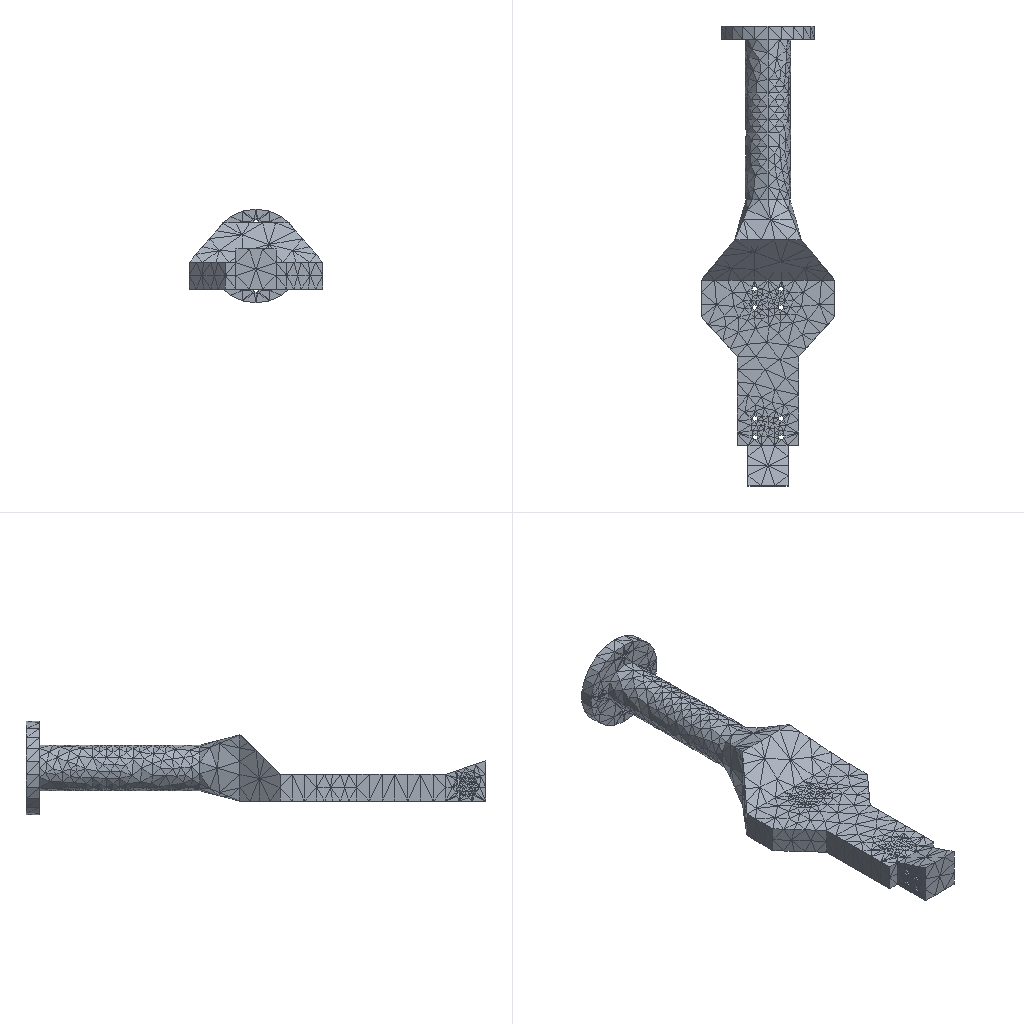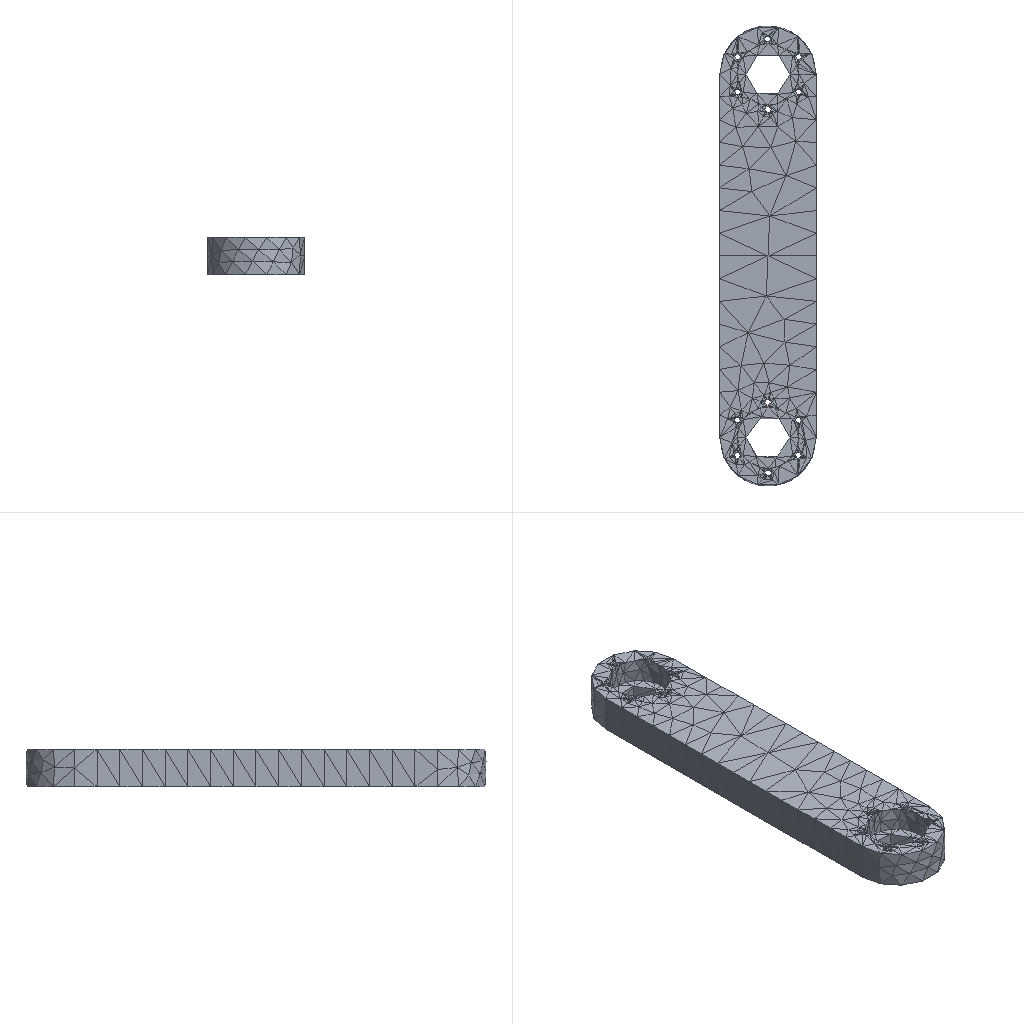Simulation study | ansys workbench
Set-up summary:
category,name,step,type,value,unit,region
solver,ansys_workbench
units,mm-N-s-tonne (MPa),,stated,"/units,MPA"
analysis,deck-1/LS1,,static
load_step,deck-1/LS1,deck-1/LS1,static,nsubst=1; time=1
analysis,deck-2/LS1,,static
load_step,deck-2/LS1,deck-2/LS1,static,nsubst=1; time=1
mesh,deck-1.dat,,nodes,16100
mesh,deck-1.dat,,elements,9885
element_type,SOLID187,,,9087,,deck-1.dat
element_type,CONTA174,,,798,,deck-1.dat
mesh,deck-2.dat,,nodes,7838
mesh,deck-2.dat,,elements,4650
element_type,SOLID187,,,4180,,deck-2.dat
element_type,SURF154,,,470,,deck-2.dat
material,Structural Steel,,E,200000,tonne s^-2 mm^-1
material,Structural Steel,,nu,0.3
material,Structural Steel,,density,7.85e-09,tonne mm^-3
material,Structural Steel,,conductivity,60.5,tonne mm s^-3 C^-1
material,Structural Steel,,specific_heat,4.34e+08,mm^2 s^-2 C^-1
material,Structural Steel,,cte,1.2e-05,C^-1
material,Structural Steel,,permeability,10000
material,Structural Steel,,resistivity,0.00017,ohm mm
material,Structural Steel,,E,200000,tonne s^-2 mm^-1
material,Structural Steel,,nu,0.3
material,Structural Steel,,density,7.85e-09,tonne mm^-3
material,Structural Steel,,conductivity,60.5,tonne mm s^-3 C^-1
material,Structural Steel,,specific_heat,4.34e+08,mm^2 s^-2 C^-1
material,Structural Steel,,cte,1.2e-05,C^-1
material,Structural Steel,,permeability,10000
material,Structural Steel,,resistivity,0.00017,ohm mm
load,,deck-1/LS1,moment,"520000 [dir=(0, 1, 0) n=3]",,all
load,Define Force Using Surface Effect Elements,deck-2/LS1,surface-effect pres face 3,-0.6729,,SURF154 #2
bc,Fixed Supports,deck-1/model,fixed,[dofs=ALL],,_FIXEDSU
bc,Fixed Supports,deck-2/model,fixed,[dofs=ALL],,_FIXEDSU
contact,contact 1,,bonded (always),element=CONTA174
named_set,______,,node,1424
named_set,_FIXEDSU,,node,1424
named_set,______,,node,2081
named_set,_FIXEDSU,,node,2081
Results summary:
result,analyses[0].index,,,1
result,analyses[0].system,,,SYS
result,analyses[0].deck,,,deck-1.dat
result,analyses[0].solve_status,,,completed
result,analyses[0].analysis_type,,,static
result,analyses[0].physics,,,mechanical
result,analyses[0].unit_system,,,"NMM: mm, ton, N, s, mV, mA, degC"
result,analyses[0].n_sets,,,1
result,analyses[0].load_steps[0].set,set=1,,1
result,analyses[0].load_steps[0].time_or_freq,set=1,,1
result,analyses[0].load_steps[0].max_displacement_magnitude,set=1,,0.01128
result,analyses[0].load_steps[0].max_von_mises_nodal,set=1,,73.33
result,analyses[0].load_steps[0].reaction_force_sum_xyz[1],set=1,,2.65462e-06
result,analyses[0].load_steps[0].reaction_force_sum_xyz[2],set=1,,-1.84965e-05
result,analyses[0].load_steps[0].reaction_force_sum_xyz[3],set=1,,6.86828e-06
result,analyses[1].index,,,2
result,analyses[1].system,,,SYS-1
result,analyses[1].deck,,,deck-2.dat
result,analyses[1].solve_status,,,completed
result,analyses[1].analysis_type,,,static
result,analyses[1].physics,,,mechanical
result,analyses[1].unit_system,,,"NMM: mm, ton, N, s, mV, mA, degC"
result,analyses[1].n_sets,,,1
result,analyses[1].load_steps[0].set,set=1,,1
result,analyses[1].load_steps[0].time_or_freq,set=1,,1
result,analyses[1].load_steps[0].max_displacement_magnitude,set=1,,0.009924
result,analyses[1].load_steps[0].max_von_mises_nodal,set=1,,110.737
result,analyses[1].load_steps[0].reaction_force_sum_xyz[1],set=1,,2.49474e-06
result,analyses[1].load_steps[0].reaction_force_sum_xyz[2],set=1,,-5.49809e-06
result,analyses[1].load_steps[0].reaction_force_sum_xyz[3],set=1,,5000